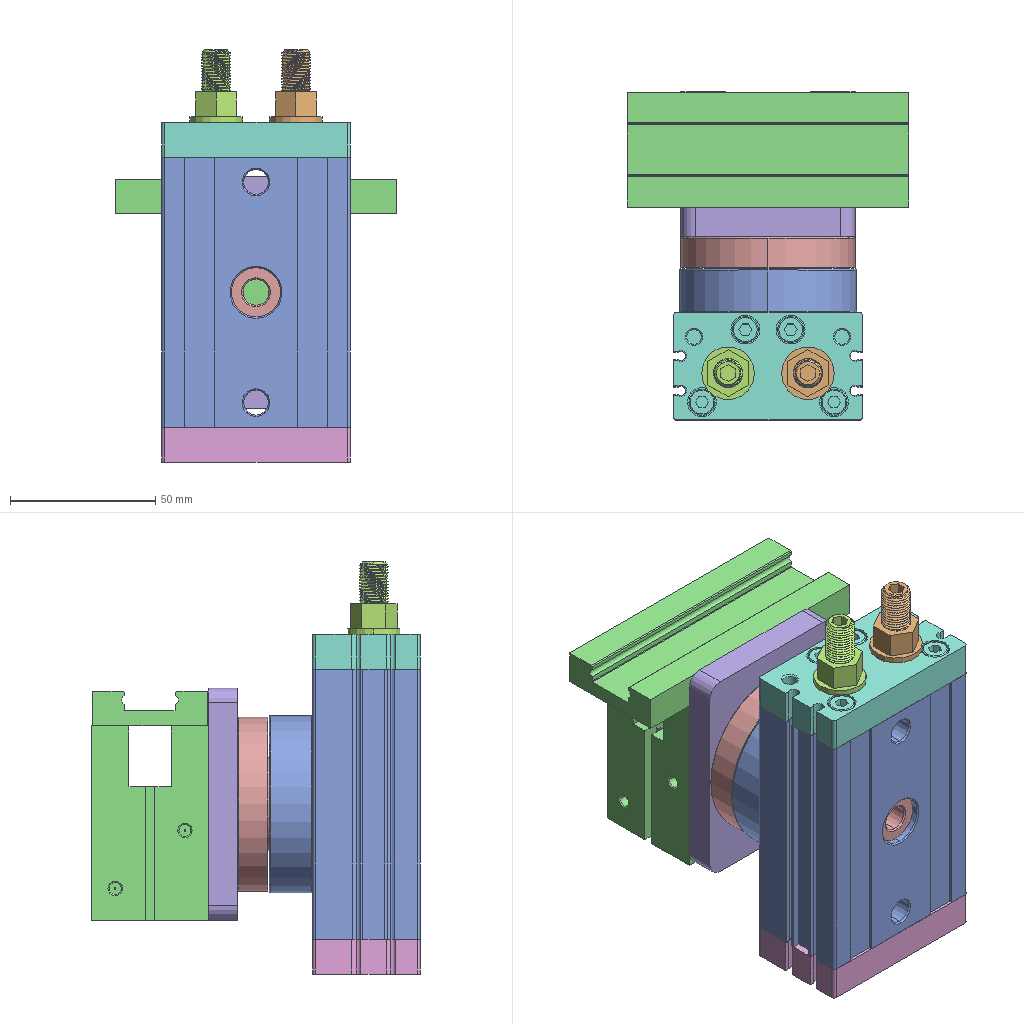Assembly | SolidWorks | 6 different items | 7 placed | box 97 x 113 x 142 mm
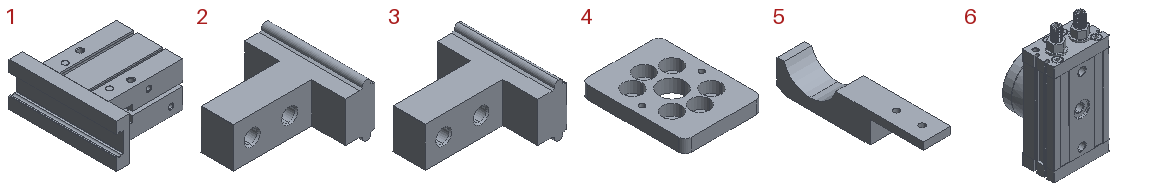Parts list (item | quantity | size | volume | features):
1 | x1 | 79 x 97 x 40 mm | 159710 mm3 | features BaseBody 1
2 | x1 | 40.2 x 37.6 x 19.68 mm | 11497 mm3 | features BaseBody 1
3 | x1 | 40.2 x 37.6 x 19.68 mm | 11497 mm3 | features BaseBody 1
4 | x1 | 60 x 80 x 10 mm | 34714 mm3 | features HoleWzd 2, CirPattern 1, Extrusion 1, Fillet 1
5 | x2 | 15 x 80 x 16 mm | 10673 mm3 | features ICE 2, Chamfer 1, Extrusion 1, HoleWzd 1
6 | x1 | 65 x 63 x 142 mm | 327794 mm3 | features ICE 19, MirrorPattern 7, Chamfer 6, Revolution 4, Fillet 3, MirrorSolid 3, CirPattern 2, DeleteBody 2, Helix 2, RevCut 2, SweepCut 2, Extrusion 1, SketchPattern 1
Mates (type | each side: item.copy, entity, surface, feature):
Coincident | 6.1 face plane Revolve4 | 4.1 face plane Boss-Extrude1
Concentric | 6.1 face cone Revolve4 | 4.1 face cylinder Boss-Extrude1
Concentric | 1.1 face cylinder Input1 | 2.1 face cylinder Input1 | 2 times
Concentric | 1.1 face cylinder Input1 | 3.1 face cylinder Input1 | 2 times
LimitDistanceDim | 2.1 face plane Input1 | 3.1 face plane Input1
Coincident | 2.1 face plane Input1 | 5.1 face plane Cut-Extrude1
Concentric | 2.1 face cylinder Input1 | 5.1 face cylinder M4 Tapped Hole1 | 2 times
Coincident | 3.1 face plane Input1 | 5.2 face plane Cut-Extrude1
Concentric | 3.1 face cylinder Input1 | 5.2 face cylinder M4 Tapped Hole1 | 2 times
Coincident | 4.1 face plane Boss-Extrude1 | 1.1 face plane Input1
Concentric | 4.1 face cylinder M5 Tapped Hole1 | 1.1 face cylinder Input1 | 2 times